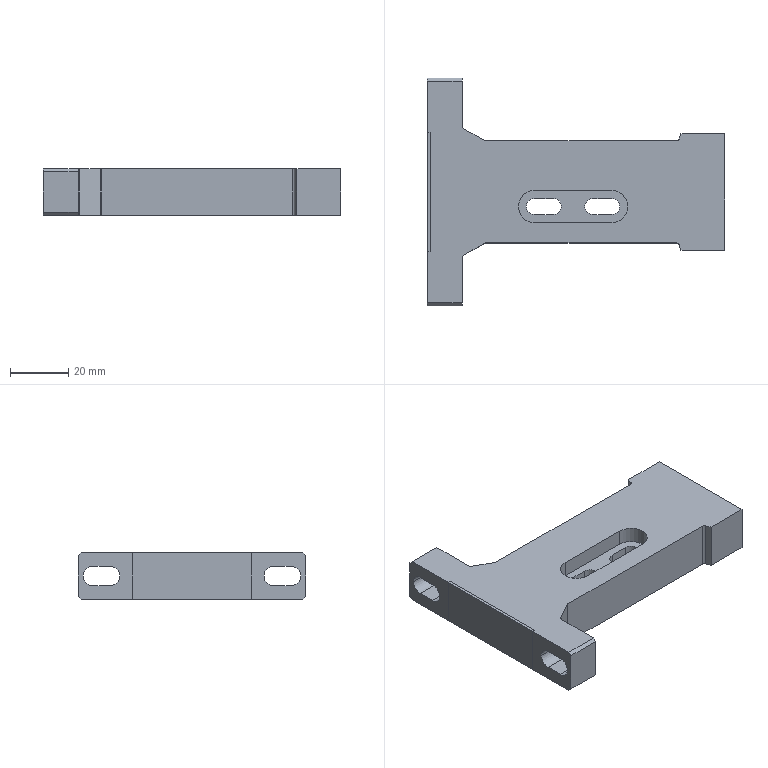NC program | NX | posted with a generic post | part box 102 x 78 x 16 mm
Whole program:
N10 G17 G21 G94 G90
(FLOOR_WALL_COPY , TOOL : D63)
N12 T01 M6
N14 G54
N16 G17 G0 G90 X-38.997 Y-85.5 B0. C0. S6500 M3
N18 G43 Z30. H1
N20 Z6.05
N22 G94 G1 Z3.05 F1250.
N24 Y-82.5
N26 Y82.5
N28 X-12.599
N30 Y-82.5
N32 X13.8
N34 Y82.5
N36 Y85.5
N38 Z6.05
N40 G0 Z30.
N42 X-38.997 Y-85.5
N44 Z5.1
N46 G1 Z2.1
N48 Y-82.5
N50 Y82.5
N52 X-12.599
N54 Y-82.5
N56 X13.8
N58 Y82.5
N60 Y85.5
N62 Z5.1
N64 G0 Z30.
N66 X-38.997 Y-85.5
N68 Z4.15
N70 G1 Z1.15
N72 Y-82.5
N74 Y82.5
N76 X-12.599
N78 Y-82.5
N80 X13.8
N82 Y82.5
N84 Y85.5
N86 Z4.15
N88 G0 Z30.
N90 X-38.997 Y-85.5
N92 Z3.2
N94 G1 Z0.2
N96 Y-82.5
N98 Y82.5
N100 X-12.599
N102 Y-82.5
N104 X13.8
N106 Y82.5
N108 Y85.5
N110 Z3.2
N112 G0 Z30.
(FLOOR_WALL_COPY_1 , TOOL : D63)
N114 X-38.997 Y-85.5
N116 Z3.
N118 G1 Z0.
N120 Y-82.5
N122 Y82.5
N124 X-12.599
N126 Y-82.5
N128 X13.8
N130 Y82.5
N132 Y85.5
N134 Z3.
N136 G0 Z30.
N138 M5
(ZLEVEL_PROFILE_COPY_COPY_1_COPY_3 , TOOL : D10JING)
N140 T11 M6
N142 G54
N144 G17 G0 G90 X9.698 Y-58.142 B0. C0. S9500 M3
N146 G43 Z30. H11
N148 Z-0.833
N150 G94 G1 X11.02 Y-57.344 F1200.
N152 G3 X11.503 Y-56.468 R1.
N154 G1 X11.501 Y-56.352
N156 X11.5 Y-50.543
N158 Y50.
N160 X11.52 Y50.449
N162 X11.501 Y50.465
N164 Y55.352
N166 X11.503 Y55.468
N168 G3 X11.02 Y56.344 R1.
N170 G1 X9.697 Y57.142
N172 G0 X9.701 Y57.156 Z-1.667
N174 G1 X11.02 Y56.359
N176 G2 X11.503 Y55.484 R1.
N178 G1 X11.5 Y55.352
N180 Y50.465
N182 X11.52 Y50.449
N184 X11.5 Y50.
N186 Y-50.543
N188 Y-56.352
N190 X11.503 Y-56.484
N192 G2 X11.02 Y-57.359 R1.
N194 G1 X9.701 Y-58.155
N196 G0 X9.704 Y-58.169 Z-2.5
N198 G1 X11.02 Y-57.375
N200 G3 X11.503 Y-56.499 R1.
N202 G1 X11.5 Y-56.352
N204 Y-50.543
N206 Y50.
N208 X11.519 Y50.435
N210 X11.5 Y50.451
N212 Y55.352
N214 X11.503 Y55.499
N216 G3 X11.02 Y56.375 R1.
N218 G1 X9.704 Y57.169
N220 G0 Z30.
N222 X5.202 Y57.142
N224 Z-0.833
N226 G1 X3.88 Y56.344
N228 G3 X3.397 Y55.468 R1.
N230 G1 X3.399 Y55.352
N232 X3.398 Y50.136
N234 X3.4 Y50.
N236 Y-50.543
N238 X3.399 Y-56.352
N240 X3.397 Y-56.468
N242 G3 X3.88 Y-57.344 R1.
N244 G1 X5.202 Y-58.142
N246 G0 X5.199 Y-58.155 Z-1.667
N248 G1 X3.88 Y-57.359
N250 G2 X3.397 Y-56.484 R1.
N252 G1 X3.4 Y-56.352
N254 Y-50.543
N256 Y50.
N258 Y55.352
N260 X3.397 Y55.484
N262 G2 X3.88 Y56.359 R1.
N264 G1 X5.199 Y57.155
N266 G0 X5.207 Y57.122 Z-2.5
N268 G1 X3.897 Y56.365
N270 G3 X3.397 Y55.499 R1.
N272 G1 X3.4 Y50.
N274 Y-50.543
N276 Y-56.352
N278 X3.397 Y-56.499
N280 G3 X3.88 Y-57.375 R1.
N282 G1 X5.196 Y-58.169
N284 G0 Z30.
N286 M5
(ZLEVEL_PROFILE_1_COPY_1_COPY , TOOL : D6A45)
N288 T07 M6
N290 G54
N292 G17 G0 G90 X0.887 Y50.941 B0. C0. S9500 M3
N294 G43 Z30. H7
N296 Z-0.5
N298 G94 G1 Z-1.5 F1000.
N300 X0.159 Y50.52
N302 G3 X-0.141 Y50.001 R0.6
N304 G1 Y-51.001
N306 G2 X-1.599 Y-52.459 R1.458
N308 G1 X-20.001
N310 G2 X-21.459 Y-51.001 R1.458
N312 G1 Y-35.999
N314 G2 X-20.5 Y-34.63 R1.457
N316 G1 X-18.959 Y-34.069
N318 Y30.815
N320 X-22.842 Y37.541
N322 X-38.001
N324 G2 X-39.459 Y38.999 R1.458
N326 G1 Y51.001
N328 G2 X-38.001 Y52.459 R1.458
N330 G1 X-20.499
N332 G2 X-19.118 Y51.459 R1.456
N334 G1 X-1.599
N336 G2 X-0.141 Y50.001 R1.458
N338 G3 X0.159 Y49.481 R0.6
N340 G1 X1.059 Y48.961
N342 Z-0.5
N344 G0 Z30.
N346 X14.013 Y-51.941
N348 Z-0.5
N350 G1 Z-1.5
N352 X14.741 Y-51.52
N354 G3 X15.041 Y-51.001 R0.6
N356 G1 Y50.001
N358 G2 X16.499 Y51.459 R1.458
N360 G1 X19.118
N362 G2 X20.499 Y52.459 R1.456
N364 G1 X38.001
N366 G2 X39.459 Y51.001 R1.458
N368 G1 Y38.999
N370 G2 X38.001 Y37.541 R1.458
N372 G1 X22.842
N374 X18.959 Y30.815
N376 Y-34.069
N378 X20.5 Y-34.63
N380 G2 X21.459 Y-35.999 R1.457
N382 G1 Y-51.001
N384 G2 X20.001 Y-52.459 R1.458
N386 G1 X16.499
N388 G2 X15.041 Y-51.001 R1.458
N390 G3 X14.741 Y-50.481 R0.6
N392 G1 X13.841 Y-49.962
N394 Z-0.5
N396 G0 Z30.
(ZLEVEL_PROFILE_1_COPY_1_COPY_COPY , TOOL : D6A45)
N398 X5.081 Y7.708
N400 Z-3.
N402 G1 Z-4.
N404 X5.991 Y7.23
N406 G3 X6.291 Y7.75 R0.6
N408 G1 Y14.25
N410 G3 X5. Y15.541 R1.291
N412 X3.709 Y14.25 R1.291
N414 G1 Y7.75
N416 G3 X5. Y6.459 R1.291
N418 X6.291 Y7.75 R1.291
N420 X5.991 Y8.27 R0.6
N422 G1 X5.091 Y8.789
N424 Z-3.
N426 G0 Z30.
N428 X5.081 Y-12.292
N430 Z-3.
N432 G1 Z-4.
N434 X5.991 Y-12.77
N436 G3 X6.291 Y-12.25 R0.6
N438 G1 Y-5.75
N440 G3 X5. Y-4.459 R1.291
N442 X3.709 Y-5.75 R1.291
N444 G1 Y-12.25
N446 G3 X5. Y-13.541 R1.291
N448 X6.291 Y-12.25 R1.291
N450 X5.991 Y-11.73 R0.6
N452 G1 X5.091 Y-11.211
N454 Z-3.
N456 G0 Z30.
N458 X1.506 Y52.716
N460 Z-3.
N462 G1 Z-4.
N464 X1.137 Y52.059
N466 G3 X1.145 Y51.459 R0.6
N468 G1 X13.755
N470 G3 X13.756 Y52.059 R0.6
N472 G1 X13.383 Y52.71
N474 Z-3.
N476 G0 Z30.
N478 X13.38 Y-53.708
N480 Z-3.
N482 G1 Z-4.
N484 X13.755 Y-53.059
N486 G3 X13.755 Y-52.459 R0.6
N488 G1 X1.145
N490 G3 X1.139 Y-53.059 R0.6
N492 G1 X1.509 Y-53.715
N494 Z-3.
N496 G0 Z30.
N498 M5
N500 M2